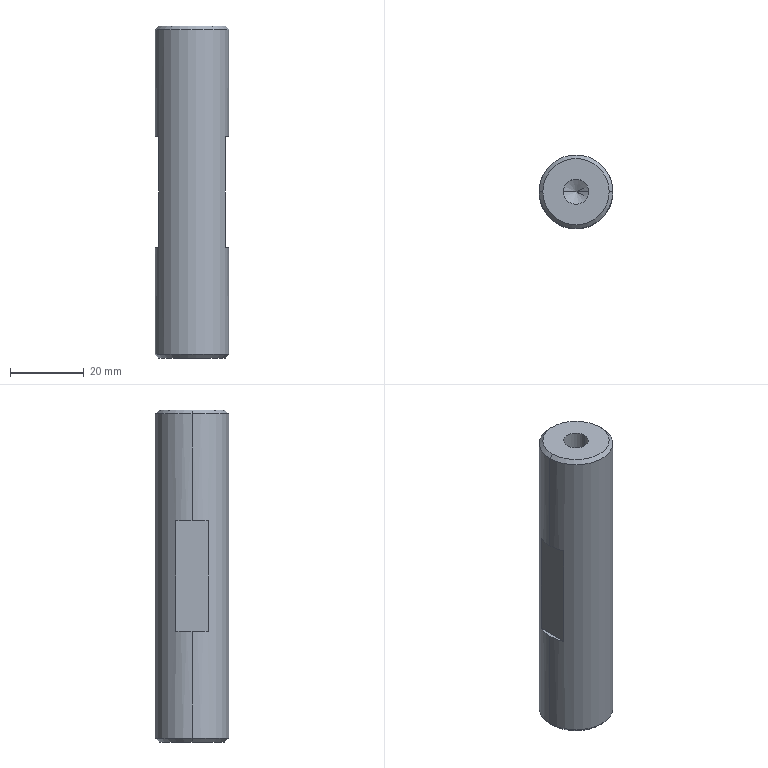Part | STEP file | 08-07 limit post | 1 solid | 22 faces | box 20 x 20 x 90 mm | volume 26377 mm3 | cone 8 | plane 8 | cylinder 6 | commonest cylinder face diameters 6.8 x4 20 x2
STEP:
#1=CARTESIAN_POINT('',(3.4,0.,19.75));
#2=VERTEX_POINT('',#1);
#3=CARTESIAN_POINT('',(-3.4,0.,19.75));
#4=VERTEX_POINT('',#3);
#5=CARTESIAN_POINT('',(0.,0.,19.75));
#6=DIRECTION('',(0.,0.,-1.));
#7=DIRECTION('',(-1.,0.,0.));
#8=AXIS2_PLACEMENT_3D('',#5,#6,#7);
#9=CIRCLE('',#8,3.4);
#10=EDGE_CURVE('',#2,#4,#9,.T.);
#11=ORIENTED_EDGE('',*,*,#10,.F.);
#12=CARTESIAN_POINT('',(3.4,0.,0.));
#13=VERTEX_POINT('',#12);
#14=CARTESIAN_POINT('',(3.4,0.,0.));
#15=DIRECTION('',(0.,0.,-1.));
#16=VECTOR('',#15,1000.);
#17=LINE('',#14,#16);
#18=EDGE_CURVE('',#2,#13,#17,.T.);
#19=ORIENTED_EDGE('',*,*,#18,.T.);
#20=CARTESIAN_POINT('',(-3.4,0.,0.));
#21=VERTEX_POINT('',#20);
#22=CARTESIAN_POINT('',(0.,0.,0.));
#23=DIRECTION('',(0.,0.,-1.));
#24=DIRECTION('',(-1.,0.,0.));
#25=AXIS2_PLACEMENT_3D('',#22,#23,#24);
#26=CIRCLE('',#25,3.4);
#27=EDGE_CURVE('',#13,#21,#26,.T.);
#28=ORIENTED_EDGE('',*,*,#27,.T.);
#29=CARTESIAN_POINT('',(-3.4,0.,0.));
#30=DIRECTION('',(0.,0.,-1.));
#31=VECTOR('',#30,1000.);
#32=LINE('',#29,#31);
#33=EDGE_CURVE('',#4,#21,#32,.T.);
#34=ORIENTED_EDGE('',*,*,#33,.F.);
#35=EDGE_LOOP('',(#11,#19,#28,#34));
#36=FACE_OUTER_BOUND('',#35,.T.);
#37=CARTESIAN_POINT('',(0.,0.,0.));
#38=DIRECTION('',(0.,0.,-1.));
#39=DIRECTION('',(-1.,0.,0.));
#40=AXIS2_PLACEMENT_3D('',#37,#38,#39);
#41=CYLINDRICAL_SURFACE('',#40,3.4);
#42=ADVANCED_FACE('',(#36),#41,.F.);
#43=CARTESIAN_POINT('',(0.,0.,21.793));
#44=VERTEX_POINT('',#43);
#45=CARTESIAN_POINT('',(-3.4,0.,19.75));
#46=DIRECTION('',(-0.8572,0.,-0.515));
#47=VECTOR('',#46,1000.);
#48=LINE('',#45,#47);
#49=EDGE_CURVE('',#44,#4,#48,.T.);
#50=ORIENTED_EDGE('',*,*,#49,.F.);
#51=CARTESIAN_POINT('',(3.4,0.,19.75));
#52=DIRECTION('',(0.8572,0.,-0.515));
#53=VECTOR('',#52,1000.);
#54=LINE('',#51,#53);
#55=EDGE_CURVE('',#44,#2,#54,.T.);
#56=ORIENTED_EDGE('',*,*,#55,.T.);
#57=ORIENTED_EDGE('',*,*,#10,.T.);
#58=EDGE_LOOP('',(#50,#56,#57));
#59=FACE_OUTER_BOUND('',#58,.T.);
#60=CARTESIAN_POINT('',(0.,0.,19.75));
#61=DIRECTION('',(0.,0.,-1.));
#62=DIRECTION('',(-1.,0.,0.));
#63=AXIS2_PLACEMENT_3D('',#60,#61,#62);
#64=CONICAL_SURFACE('',#63,3.4,1.03);
#65=ADVANCED_FACE('',(#59),#64,.F.);
#66=CARTESIAN_POINT('',(-3.4,0.,70.25));
#67=VERTEX_POINT('',#66);
#68=CARTESIAN_POINT('',(3.4,0.,70.25));
#69=VERTEX_POINT('',#68);
#70=CARTESIAN_POINT('',(0.,0.,70.25));
#71=DIRECTION('',(0.,0.,1.));
#72=DIRECTION('',(1.,0.,0.));
#73=AXIS2_PLACEMENT_3D('',#70,#71,#72);
#74=CIRCLE('',#73,3.4);
#75=EDGE_CURVE('',#67,#69,#74,.T.);
#76=ORIENTED_EDGE('',*,*,#75,.F.);
#77=CARTESIAN_POINT('',(-3.4,0.,90.));
#78=VERTEX_POINT('',#77);
#79=CARTESIAN_POINT('',(-3.4,0.,90.));
#80=DIRECTION('',(0.,0.,1.));
#81=VECTOR('',#80,1000.);
#82=LINE('',#79,#81);
#83=EDGE_CURVE('',#67,#78,#82,.T.);
#84=ORIENTED_EDGE('',*,*,#83,.T.);
#85=CARTESIAN_POINT('',(3.4,0.,90.));
#86=VERTEX_POINT('',#85);
#87=CARTESIAN_POINT('',(0.,0.,90.));
#88=DIRECTION('',(0.,0.,1.));
#89=DIRECTION('',(1.,0.,0.));
#90=AXIS2_PLACEMENT_3D('',#87,#88,#89);
#91=CIRCLE('',#90,3.4);
#92=EDGE_CURVE('',#78,#86,#91,.T.);
#93=ORIENTED_EDGE('',*,*,#92,.T.);
#94=CARTESIAN_POINT('',(3.4,0.,90.));
#95=DIRECTION('',(0.,0.,1.));
#96=VECTOR('',#95,1000.);
#97=LINE('',#94,#96);
#98=EDGE_CURVE('',#69,#86,#97,.T.);
#99=ORIENTED_EDGE('',*,*,#98,.F.);
#100=EDGE_LOOP('',(#76,#84,#93,#99));
#101=FACE_OUTER_BOUND('',#100,.T.);
#102=CARTESIAN_POINT('',(0.,0.,90.));
#103=DIRECTION('',(0.,0.,1.));
#104=DIRECTION('',(1.,0.,0.));
#105=AXIS2_PLACEMENT_3D('',#102,#103,#104);
#106=CYLINDRICAL_SURFACE('',#105,3.4);
#107=ADVANCED_FACE('',(#101),#106,.F.);
#108=CARTESIAN_POINT('',(0.,0.,68.207));
#109=VERTEX_POINT('',#108);
#110=CARTESIAN_POINT('',(3.4,0.,70.25));
#111=DIRECTION('',(0.8572,0.,0.515));
#112=VECTOR('',#111,1000.);
#113=LINE('',#110,#112);
#114=EDGE_CURVE('',#109,#69,#113,.T.);
#115=ORIENTED_EDGE('',*,*,#114,.F.);
#116=CARTESIAN_POINT('',(-3.4,0.,70.25));
#117=DIRECTION('',(-0.8572,0.,0.515));
#118=VECTOR('',#117,1000.);
#119=LINE('',#116,#118);
#120=EDGE_CURVE('',#109,#67,#119,.T.);
#121=ORIENTED_EDGE('',*,*,#120,.T.);
#122=ORIENTED_EDGE('',*,*,#75,.T.);
#123=EDGE_LOOP('',(#115,#121,#122));
#124=FACE_OUTER_BOUND('',#123,.T.);
#125=CARTESIAN_POINT('',(0.,0.,70.25));
#126=DIRECTION('',(0.,0.,1.));
#127=DIRECTION('',(1.,0.,0.));
#128=AXIS2_PLACEMENT_3D('',#125,#126,#127);
#129=CONICAL_SURFACE('',#128,3.4,1.03);
#130=ADVANCED_FACE('',(#124),#129,.F.);
#131=CARTESIAN_POINT('',(9.,0.,90.));
#132=VERTEX_POINT('',#131);
#133=CARTESIAN_POINT('',(-9.,0.,90.));
#134=VERTEX_POINT('',#133);
#135=CARTESIAN_POINT('',(0.,0.,90.));
#136=DIRECTION('',(0.,0.,1.));
#137=DIRECTION('',(1.,0.,0.));
#138=AXIS2_PLACEMENT_3D('',#135,#136,#137);
#139=CIRCLE('',#138,9.);
#140=EDGE_CURVE('',#132,#134,#139,.T.);
#141=ORIENTED_EDGE('',*,*,#140,.F.);
#142=CARTESIAN_POINT('',(10.,0.,89.));
#143=VERTEX_POINT('',#142);
#144=CARTESIAN_POINT('',(9.,0.,90.));
#145=DIRECTION('',(0.7071,0.,-0.7071));
#146=VECTOR('',#145,1000.);
#147=LINE('',#144,#146);
#148=EDGE_CURVE('',#132,#143,#147,.T.);
#149=ORIENTED_EDGE('',*,*,#148,.T.);
#150=CARTESIAN_POINT('',(-10.,0.,89.));
#151=VERTEX_POINT('',#150);
#152=CARTESIAN_POINT('',(0.,0.,89.));
#153=DIRECTION('',(0.,0.,-1.));
#154=DIRECTION('',(1.,0.,0.));
#155=AXIS2_PLACEMENT_3D('',#152,#153,#154);
#156=CIRCLE('',#155,10.);
#157=EDGE_CURVE('',#151,#143,#156,.T.);
#158=ORIENTED_EDGE('',*,*,#157,.F.);
#159=CARTESIAN_POINT('',(-9.,0.,90.));
#160=DIRECTION('',(-0.7071,0.,-0.7071));
#161=VECTOR('',#160,1000.);
#162=LINE('',#159,#161);
#163=EDGE_CURVE('',#134,#151,#162,.T.);
#164=ORIENTED_EDGE('',*,*,#163,.F.);
#165=EDGE_LOOP('',(#141,#149,#158,#164));
#166=FACE_OUTER_BOUND('',#165,.T.);
#167=CARTESIAN_POINT('',(0.,0.,90.));
#168=DIRECTION('',(0.,0.,-1.));
#169=DIRECTION('',(-1.,0.,0.));
#170=AXIS2_PLACEMENT_3D('',#167,#168,#169);
#171=CONICAL_SURFACE('',#170,9.,0.7854);
#172=ADVANCED_FACE('',(#166),#171,.T.);
#173=CARTESIAN_POINT('',(-9.,0.,0.));
#174=VERTEX_POINT('',#173);
#175=CARTESIAN_POINT('',(9.,0.,0.));
#176=VERTEX_POINT('',#175);
#177=CARTESIAN_POINT('',(0.,0.,0.));
#178=DIRECTION('',(0.,0.,-1.));
#179=DIRECTION('',(1.,0.,0.));
#180=AXIS2_PLACEMENT_3D('',#177,#178,#179);
#181=CIRCLE('',#180,9.);
#182=EDGE_CURVE('',#174,#176,#181,.T.);
#183=ORIENTED_EDGE('',*,*,#182,.F.);
#184=CARTESIAN_POINT('',(-10.,0.,1.));
#185=VERTEX_POINT('',#184);
#186=CARTESIAN_POINT('',(-10.,0.,1.));
#187=DIRECTION('',(-0.7071,0.,0.7071));
#188=VECTOR('',#187,1000.);
#189=LINE('',#186,#188);
#190=EDGE_CURVE('',#174,#185,#189,.T.);
#191=ORIENTED_EDGE('',*,*,#190,.T.);
#192=CARTESIAN_POINT('',(10.,0.,1.));
#193=VERTEX_POINT('',#192);
#194=CARTESIAN_POINT('',(0.,0.,1.));
#195=DIRECTION('',(0.,0.,1.));
#196=DIRECTION('',(1.,0.,0.));
#197=AXIS2_PLACEMENT_3D('',#194,#195,#196);
#198=CIRCLE('',#197,10.);
#199=EDGE_CURVE('',#193,#185,#198,.T.);
#200=ORIENTED_EDGE('',*,*,#199,.F.);
#201=CARTESIAN_POINT('',(10.,0.,1.));
#202=DIRECTION('',(0.7071,0.,0.7071));
#203=VECTOR('',#202,1000.);
#204=LINE('',#201,#203);
#205=EDGE_CURVE('',#176,#193,#204,.T.);
#206=ORIENTED_EDGE('',*,*,#205,.F.);
#207=EDGE_LOOP('',(#183,#191,#200,#206));
#208=FACE_OUTER_BOUND('',#207,.T.);
#209=CARTESIAN_POINT('',(0.,0.,1.));
#210=DIRECTION('',(0.,0.,1.));
#211=DIRECTION('',(1.,0.,0.));
#212=AXIS2_PLACEMENT_3D('',#209,#210,#211);
#213=CONICAL_SURFACE('',#212,10.,0.7854);
#214=ADVANCED_FACE('',(#208),#213,.T.);
#215=ORIENTED_EDGE('',*,*,#157,.T.);
#216=CARTESIAN_POINT('',(10.,0.,60.));
#217=VERTEX_POINT('',#216);
#218=CARTESIAN_POINT('',(10.,0.,90.));
#219=DIRECTION('',(0.,0.,-1.));
#220=VECTOR('',#219,1000.);
#221=LINE('',#218,#220);
#222=EDGE_CURVE('',#143,#217,#221,.T.);
#223=ORIENTED_EDGE('',*,*,#222,.T.);
#224=CARTESIAN_POINT('',(9.,4.359,60.));
#225=VERTEX_POINT('',#224);
#226=CARTESIAN_POINT('',(0.,0.,60.));
#227=DIRECTION('',(0.,0.,1.));
#228=DIRECTION('',(1.,0.,0.));
#229=AXIS2_PLACEMENT_3D('',#226,#227,#228);
#230=CIRCLE('',#229,10.);
#231=EDGE_CURVE('',#217,#225,#230,.T.);
#232=ORIENTED_EDGE('',*,*,#231,.T.);
#233=CARTESIAN_POINT('',(9.,4.359,30.));
#234=VERTEX_POINT('',#233);
#235=CARTESIAN_POINT('',(9.,4.359,90.));
#236=DIRECTION('',(0.,0.,-1.));
#237=VECTOR('',#236,1000.);
#238=LINE('',#235,#237);
#239=EDGE_CURVE('',#225,#234,#238,.T.);
#240=ORIENTED_EDGE('',*,*,#239,.T.);
#241=CARTESIAN_POINT('',(10.,0.,30.));
#242=VERTEX_POINT('',#241);
#243=CARTESIAN_POINT('',(0.,0.,30.));
#244=DIRECTION('',(0.,0.,-1.));
#245=DIRECTION('',(-1.,0.,0.));
#246=AXIS2_PLACEMENT_3D('',#243,#244,#245);
#247=CIRCLE('',#246,10.);
#248=EDGE_CURVE('',#234,#242,#247,.T.);
#249=ORIENTED_EDGE('',*,*,#248,.T.);
#250=CARTESIAN_POINT('',(10.,0.,90.));
#251=DIRECTION('',(0.,0.,-1.));
#252=VECTOR('',#251,1000.);
#253=LINE('',#250,#252);
#254=EDGE_CURVE('',#242,#193,#253,.T.);
#255=ORIENTED_EDGE('',*,*,#254,.T.);
#256=ORIENTED_EDGE('',*,*,#199,.T.);
#257=CARTESIAN_POINT('',(-10.,0.,30.));
#258=VERTEX_POINT('',#257);
#259=CARTESIAN_POINT('',(-10.,0.,90.));
#260=DIRECTION('',(0.,0.,-1.));
#261=VECTOR('',#260,1000.);
#262=LINE('',#259,#261);
#263=EDGE_CURVE('',#258,#185,#262,.T.);
#264=ORIENTED_EDGE('',*,*,#263,.F.);
#265=CARTESIAN_POINT('',(-9.,4.359,30.));
#266=VERTEX_POINT('',#265);
#267=CARTESIAN_POINT('',(0.,0.,30.));
#268=DIRECTION('',(0.,0.,-1.));
#269=DIRECTION('',(-1.,0.,0.));
#270=AXIS2_PLACEMENT_3D('',#267,#268,#269);
#271=CIRCLE('',#270,10.);
#272=EDGE_CURVE('',#258,#266,#271,.T.);
#273=ORIENTED_EDGE('',*,*,#272,.T.);
#274=CARTESIAN_POINT('',(-9.,4.359,60.));
#275=VERTEX_POINT('',#274);
#276=CARTESIAN_POINT('',(-9.,4.359,90.));
#277=DIRECTION('',(0.,0.,1.));
#278=VECTOR('',#277,1000.);
#279=LINE('',#276,#278);
#280=EDGE_CURVE('',#266,#275,#279,.T.);
#281=ORIENTED_EDGE('',*,*,#280,.T.);
#282=CARTESIAN_POINT('',(-10.,0.,60.));
#283=VERTEX_POINT('',#282);
#284=CARTESIAN_POINT('',(0.,0.,60.));
#285=DIRECTION('',(0.,0.,1.));
#286=DIRECTION('',(1.,0.,0.));
#287=AXIS2_PLACEMENT_3D('',#284,#285,#286);
#288=CIRCLE('',#287,10.);
#289=EDGE_CURVE('',#275,#283,#288,.T.);
#290=ORIENTED_EDGE('',*,*,#289,.T.);
#291=CARTESIAN_POINT('',(-10.,0.,90.));
#292=DIRECTION('',(0.,0.,-1.));
#293=VECTOR('',#292,1000.);
#294=LINE('',#291,#293);
#295=EDGE_CURVE('',#151,#283,#294,.T.);
#296=ORIENTED_EDGE('',*,*,#295,.F.);
#297=EDGE_LOOP('',(#215,#223,#232,#240,#249,#255,#256,#264,#273,#281,#290,#296));
#298=FACE_OUTER_BOUND('',#297,.T.);
#299=CARTESIAN_POINT('',(0.,0.,90.));
#300=DIRECTION('',(0.,0.,-1.));
#301=DIRECTION('',(-1.,0.,0.));
#302=AXIS2_PLACEMENT_3D('',#299,#300,#301);
#303=CYLINDRICAL_SURFACE('',#302,10.);
#304=ADVANCED_FACE('',(#298),#303,.T.);
#305=ORIENTED_EDGE('',*,*,#222,.F.);
#306=CARTESIAN_POINT('',(0.,0.,89.));
#307=DIRECTION('',(0.,0.,-1.));
#308=DIRECTION('',(1.,0.,0.));
#309=AXIS2_PLACEMENT_3D('',#306,#307,#308);
#310=CIRCLE('',#309,10.);
#311=EDGE_CURVE('',#143,#151,#310,.T.);
#312=ORIENTED_EDGE('',*,*,#311,.T.);
#313=ORIENTED_EDGE('',*,*,#295,.T.);
#314=CARTESIAN_POINT('',(-9.,-4.359,60.));
#315=VERTEX_POINT('',#314);
#316=CARTESIAN_POINT('',(0.,0.,60.));
#317=DIRECTION('',(0.,0.,1.));
#318=DIRECTION('',(1.,0.,0.));
#319=AXIS2_PLACEMENT_3D('',#316,#317,#318);
#320=CIRCLE('',#319,10.);
#321=EDGE_CURVE('',#283,#315,#320,.T.);
#322=ORIENTED_EDGE('',*,*,#321,.T.);
#323=CARTESIAN_POINT('',(-9.,-4.359,30.));
#324=VERTEX_POINT('',#323);
#325=CARTESIAN_POINT('',(-9.,-4.359,90.));
#326=DIRECTION('',(0.,0.,-1.));
#327=VECTOR('',#326,1000.);
#328=LINE('',#325,#327);
#329=EDGE_CURVE('',#315,#324,#328,.T.);
#330=ORIENTED_EDGE('',*,*,#329,.T.);
#331=CARTESIAN_POINT('',(0.,0.,30.));
#332=DIRECTION('',(0.,0.,-1.));
#333=DIRECTION('',(-1.,0.,0.));
#334=AXIS2_PLACEMENT_3D('',#331,#332,#333);
#335=CIRCLE('',#334,10.);
#336=EDGE_CURVE('',#324,#258,#335,.T.);
#337=ORIENTED_EDGE('',*,*,#336,.T.);
#338=ORIENTED_EDGE('',*,*,#263,.T.);
#339=CARTESIAN_POINT('',(0.,0.,1.));
#340=DIRECTION('',(0.,0.,1.));
#341=DIRECTION('',(1.,0.,0.));
#342=AXIS2_PLACEMENT_3D('',#339,#340,#341);
#343=CIRCLE('',#342,10.);
#344=EDGE_CURVE('',#185,#193,#343,.T.);
#345=ORIENTED_EDGE('',*,*,#344,.T.);
#346=ORIENTED_EDGE('',*,*,#254,.F.);
#347=CARTESIAN_POINT('',(9.,-4.359,30.));
#348=VERTEX_POINT('',#347);
#349=CARTESIAN_POINT('',(0.,0.,30.));
#350=DIRECTION('',(0.,0.,-1.));
#351=DIRECTION('',(-1.,0.,0.));
#352=AXIS2_PLACEMENT_3D('',#349,#350,#351);
#353=CIRCLE('',#352,10.);
#354=EDGE_CURVE('',#242,#348,#353,.T.);
#355=ORIENTED_EDGE('',*,*,#354,.T.);
#356=CARTESIAN_POINT('',(9.,-4.359,60.));
#357=VERTEX_POINT('',#356);
#358=CARTESIAN_POINT('',(9.,-4.359,90.));
#359=DIRECTION('',(0.,0.,1.));
#360=VECTOR('',#359,1000.);
#361=LINE('',#358,#360);
#362=EDGE_CURVE('',#348,#357,#361,.T.);
#363=ORIENTED_EDGE('',*,*,#362,.T.);
#364=CARTESIAN_POINT('',(0.,0.,60.));
#365=DIRECTION('',(0.,0.,1.));
#366=DIRECTION('',(1.,0.,0.));
#367=AXIS2_PLACEMENT_3D('',#364,#365,#366);
#368=CIRCLE('',#367,10.);
#369=EDGE_CURVE('',#357,#217,#368,.T.);
#370=ORIENTED_EDGE('',*,*,#369,.T.);
#371=EDGE_LOOP('',(#305,#312,#313,#322,#330,#337,#338,#345,#346,#355,#363,#370));
#372=FACE_OUTER_BOUND('',#371,.T.);
#373=CARTESIAN_POINT('',(0.,0.,90.));
#374=DIRECTION('',(0.,0.,-1.));
#375=DIRECTION('',(-1.,0.,0.));
#376=AXIS2_PLACEMENT_3D('',#373,#374,#375);
#377=CYLINDRICAL_SURFACE('',#376,10.);
#378=ADVANCED_FACE('',(#372),#377,.T.);
#379=CARTESIAN_POINT('',(0.,0.,90.));
#380=DIRECTION('',(0.,0.,1.));
#381=DIRECTION('',(1.,0.,0.));
#382=AXIS2_PLACEMENT_3D('',#379,#380,#381);
#383=CIRCLE('',#382,3.4);
#384=EDGE_CURVE('',#86,#78,#383,.T.);
#385=ORIENTED_EDGE('',*,*,#384,.F.);
#386=ORIENTED_EDGE('',*,*,#92,.F.);
#387=EDGE_LOOP('',(#385,#386));
#388=FACE_BOUND('',#387,.T.);
#389=CARTESIAN_POINT('',(0.,0.,90.));
#390=DIRECTION('',(0.,0.,1.));
#391=DIRECTION('',(1.,0.,0.));
#392=AXIS2_PLACEMENT_3D('',#389,#390,#391);
#393=CIRCLE('',#392,9.);
#394=EDGE_CURVE('',#134,#132,#393,.T.);
#395=ORIENTED_EDGE('',*,*,#394,.T.);
#396=ORIENTED_EDGE('',*,*,#140,.T.);
#397=EDGE_LOOP('',(#395,#396));
#398=FACE_OUTER_BOUND('',#397,.T.);
#399=CARTESIAN_POINT('',(0.,0.,90.));
#400=DIRECTION('',(0.,0.,1.));
#401=DIRECTION('',(1.,0.,0.));
#402=AXIS2_PLACEMENT_3D('',#399,#400,#401);
#403=PLANE('',#402);
#404=ADVANCED_FACE('',(#388,#398),#403,.T.);
#405=CARTESIAN_POINT('',(0.,0.,0.));
#406=DIRECTION('',(0.,0.,-1.));
#407=DIRECTION('',(-1.,0.,0.));
#408=AXIS2_PLACEMENT_3D('',#405,#406,#407);
#409=CIRCLE('',#408,3.4);
#410=EDGE_CURVE('',#21,#13,#409,.T.);
#411=ORIENTED_EDGE('',*,*,#410,.F.);
#412=ORIENTED_EDGE('',*,*,#27,.F.);
#413=EDGE_LOOP('',(#411,#412));
#414=FACE_BOUND('',#413,.T.);
#415=CARTESIAN_POINT('',(0.,0.,0.));
#416=DIRECTION('',(0.,0.,-1.));
#417=DIRECTION('',(1.,0.,0.));
#418=AXIS2_PLACEMENT_3D('',#415,#416,#417);
#419=CIRCLE('',#418,9.);
#420=EDGE_CURVE('',#176,#174,#419,.T.);
#421=ORIENTED_EDGE('',*,*,#420,.T.);
#422=ORIENTED_EDGE('',*,*,#182,.T.);
#423=EDGE_LOOP('',(#421,#422));
#424=FACE_OUTER_BOUND('',#423,.T.);
#425=CARTESIAN_POINT('',(0.,0.,0.));
#426=DIRECTION('',(0.,0.,1.));
#427=DIRECTION('',(1.,0.,0.));
#428=AXIS2_PLACEMENT_3D('',#425,#426,#427);
#429=PLANE('',#428);
#430=ADVANCED_FACE('',(#414,#424),#429,.F.);
#431=ORIENTED_EDGE('',*,*,#190,.F.);
#432=ORIENTED_EDGE('',*,*,#420,.F.);
#433=ORIENTED_EDGE('',*,*,#205,.T.);
#434=ORIENTED_EDGE('',*,*,#344,.F.);
#435=EDGE_LOOP('',(#431,#432,#433,#434));
#436=FACE_OUTER_BOUND('',#435,.T.);
#437=CARTESIAN_POINT('',(0.,0.,1.));
#438=DIRECTION('',(0.,0.,1.));
#439=DIRECTION('',(1.,0.,0.));
#440=AXIS2_PLACEMENT_3D('',#437,#438,#439);
#441=CONICAL_SURFACE('',#440,10.,0.7854);
#442=ADVANCED_FACE('',(#436),#441,.T.);
#443=ORIENTED_EDGE('',*,*,#148,.F.);
#444=ORIENTED_EDGE('',*,*,#394,.F.);
#445=ORIENTED_EDGE('',*,*,#163,.T.);
#446=ORIENTED_EDGE('',*,*,#311,.F.);
#447=EDGE_LOOP('',(#443,#444,#445,#446));
#448=FACE_OUTER_BOUND('',#447,.T.);
#449=CARTESIAN_POINT('',(0.,0.,90.));
#450=DIRECTION('',(0.,0.,-1.));
#451=DIRECTION('',(-1.,0.,0.));
#452=AXIS2_PLACEMENT_3D('',#449,#450,#451);
#453=CONICAL_SURFACE('',#452,9.,0.7854);
#454=ADVANCED_FACE('',(#448),#453,.T.);
#455=ORIENTED_EDGE('',*,*,#120,.F.);
#456=ORIENTED_EDGE('',*,*,#114,.T.);
#457=CARTESIAN_POINT('',(0.,0.,70.25));
#458=DIRECTION('',(0.,0.,1.));
#459=DIRECTION('',(1.,0.,0.));
#460=AXIS2_PLACEMENT_3D('',#457,#458,#459);
#461=CIRCLE('',#460,3.4);
#462=EDGE_CURVE('',#69,#67,#461,.T.);
#463=ORIENTED_EDGE('',*,*,#462,.T.);
#464=EDGE_LOOP('',(#455,#456,#463));
#465=FACE_OUTER_BOUND('',#464,.T.);
#466=CARTESIAN_POINT('',(0.,0.,70.25));
#467=DIRECTION('',(0.,0.,1.));
#468=DIRECTION('',(1.,0.,0.));
#469=AXIS2_PLACEMENT_3D('',#466,#467,#468);
#470=CONICAL_SURFACE('',#469,3.4,1.03);
#471=ADVANCED_FACE('',(#465),#470,.F.);
#472=ORIENTED_EDGE('',*,*,#83,.F.);
#473=ORIENTED_EDGE('',*,*,#462,.F.);
#474=ORIENTED_EDGE('',*,*,#98,.T.);
#475=ORIENTED_EDGE('',*,*,#384,.T.);
#476=EDGE_LOOP('',(#472,#473,#474,#475));
#477=FACE_OUTER_BOUND('',#476,.T.);
#478=CARTESIAN_POINT('',(0.,0.,90.));
#479=DIRECTION('',(0.,0.,1.));
#480=DIRECTION('',(1.,0.,0.));
#481=AXIS2_PLACEMENT_3D('',#478,#479,#480);
#482=CYLINDRICAL_SURFACE('',#481,3.4);
#483=ADVANCED_FACE('',(#477),#482,.F.);
#484=ORIENTED_EDGE('',*,*,#55,.F.);
#485=ORIENTED_EDGE('',*,*,#49,.T.);
#486=CARTESIAN_POINT('',(0.,0.,19.75));
#487=DIRECTION('',(0.,0.,-1.));
#488=DIRECTION('',(-1.,0.,0.));
#489=AXIS2_PLACEMENT_3D('',#486,#487,#488);
#490=CIRCLE('',#489,3.4);
#491=EDGE_CURVE('',#4,#2,#490,.T.);
#492=ORIENTED_EDGE('',*,*,#491,.T.);
#493=EDGE_LOOP('',(#484,#485,#492));
#494=FACE_OUTER_BOUND('',#493,.T.);
#495=CARTESIAN_POINT('',(0.,0.,19.75));
#496=DIRECTION('',(0.,0.,-1.));
#497=DIRECTION('',(-1.,0.,0.));
#498=AXIS2_PLACEMENT_3D('',#495,#496,#497);
#499=CONICAL_SURFACE('',#498,3.4,1.03);
#500=ADVANCED_FACE('',(#494),#499,.F.);
#501=ORIENTED_EDGE('',*,*,#18,.F.);
#502=ORIENTED_EDGE('',*,*,#491,.F.);
#503=ORIENTED_EDGE('',*,*,#33,.T.);
#504=ORIENTED_EDGE('',*,*,#410,.T.);
#505=EDGE_LOOP('',(#501,#502,#503,#504));
#506=FACE_OUTER_BOUND('',#505,.T.);
#507=CARTESIAN_POINT('',(0.,0.,0.));
#508=DIRECTION('',(0.,0.,-1.));
#509=DIRECTION('',(-1.,0.,0.));
#510=AXIS2_PLACEMENT_3D('',#507,#508,#509);
#511=CYLINDRICAL_SURFACE('',#510,3.4);
#512=ADVANCED_FACE('',(#506),#511,.F.);
#513=CARTESIAN_POINT('',(9.,-5.,60.));
#514=DIRECTION('',(0.,1.,0.));
#515=VECTOR('',#514,1000.);
#516=LINE('',#513,#515);
#517=EDGE_CURVE('',#357,#225,#516,.T.);
#518=ORIENTED_EDGE('',*,*,#517,.F.);
#519=ORIENTED_EDGE('',*,*,#362,.F.);
#520=CARTESIAN_POINT('',(9.,-5.,30.));
#521=DIRECTION('',(0.,1.,0.));
#522=VECTOR('',#521,1000.);
#523=LINE('',#520,#522);
#524=EDGE_CURVE('',#348,#234,#523,.T.);
#525=ORIENTED_EDGE('',*,*,#524,.T.);
#526=ORIENTED_EDGE('',*,*,#239,.F.);
#527=EDGE_LOOP('',(#518,#519,#525,#526));
#528=FACE_OUTER_BOUND('',#527,.T.);
#529=CARTESIAN_POINT('',(9.,-5.,30.));
#530=DIRECTION('',(-1.,0.,0.));
#531=DIRECTION('',(0.,0.,1.));
#532=AXIS2_PLACEMENT_3D('',#529,#530,#531);
#533=PLANE('',#532);
#534=ADVANCED_FACE('',(#528),#533,.F.);
#535=ORIENTED_EDGE('',*,*,#524,.F.);
#536=ORIENTED_EDGE('',*,*,#354,.F.);
#537=ORIENTED_EDGE('',*,*,#248,.F.);
#538=EDGE_LOOP('',(#535,#536,#537));
#539=FACE_OUTER_BOUND('',#538,.T.);
#540=CARTESIAN_POINT('',(9.,-5.,30.));
#541=DIRECTION('',(0.,0.,-1.));
#542=DIRECTION('',(-1.,0.,0.));
#543=AXIS2_PLACEMENT_3D('',#540,#541,#542);
#544=PLANE('',#543);
#545=ADVANCED_FACE('',(#539),#544,.F.);
#546=ORIENTED_EDGE('',*,*,#517,.T.);
#547=ORIENTED_EDGE('',*,*,#231,.F.);
#548=ORIENTED_EDGE('',*,*,#369,.F.);
#549=EDGE_LOOP('',(#546,#547,#548));
#550=FACE_OUTER_BOUND('',#549,.T.);
#551=CARTESIAN_POINT('',(9.,-5.,60.));
#552=DIRECTION('',(0.,0.,1.));
#553=DIRECTION('',(1.,0.,0.));
#554=AXIS2_PLACEMENT_3D('',#551,#552,#553);
#555=PLANE('',#554);
#556=ADVANCED_FACE('',(#550),#555,.F.);
#557=CARTESIAN_POINT('',(-9.,-5.,30.));
#558=DIRECTION('',(0.,1.,0.));
#559=VECTOR('',#558,1000.);
#560=LINE('',#557,#559);
#561=EDGE_CURVE('',#324,#266,#560,.T.);
#562=ORIENTED_EDGE('',*,*,#561,.T.);
#563=ORIENTED_EDGE('',*,*,#272,.F.);
#564=ORIENTED_EDGE('',*,*,#336,.F.);
#565=EDGE_LOOP('',(#562,#563,#564));
#566=FACE_OUTER_BOUND('',#565,.T.);
#567=CARTESIAN_POINT('',(-9.,-5.,30.));
#568=DIRECTION('',(0.,0.,-1.));
#569=DIRECTION('',(-1.,0.,0.));
#570=AXIS2_PLACEMENT_3D('',#567,#568,#569);
#571=PLANE('',#570);
#572=ADVANCED_FACE('',(#566),#571,.F.);
#573=CARTESIAN_POINT('',(-9.,-5.,60.));
#574=DIRECTION('',(0.,1.,0.));
#575=VECTOR('',#574,1000.);
#576=LINE('',#573,#575);
#577=EDGE_CURVE('',#315,#275,#576,.T.);
#578=ORIENTED_EDGE('',*,*,#577,.T.);
#579=ORIENTED_EDGE('',*,*,#280,.F.);
#580=ORIENTED_EDGE('',*,*,#561,.F.);
#581=ORIENTED_EDGE('',*,*,#329,.F.);
#582=EDGE_LOOP('',(#578,#579,#580,#581));
#583=FACE_OUTER_BOUND('',#582,.T.);
#584=CARTESIAN_POINT('',(-9.,-5.,30.));
#585=DIRECTION('',(1.,0.,0.));
#586=DIRECTION('',(0.,0.,-1.));
#587=AXIS2_PLACEMENT_3D('',#584,#585,#586);
#588=PLANE('',#587);
#589=ADVANCED_FACE('',(#583),#588,.F.);
#590=ORIENTED_EDGE('',*,*,#577,.F.);
#591=ORIENTED_EDGE('',*,*,#321,.F.);
#592=ORIENTED_EDGE('',*,*,#289,.F.);
#593=EDGE_LOOP('',(#590,#591,#592));
#594=FACE_OUTER_BOUND('',#593,.T.);
#595=CARTESIAN_POINT('',(-9.,-5.,60.));
#596=DIRECTION('',(0.,0.,1.));
#597=DIRECTION('',(1.,0.,0.));
#598=AXIS2_PLACEMENT_3D('',#595,#596,#597);
#599=PLANE('',#598);
#600=ADVANCED_FACE('',(#594),#599,.F.);
#601=CLOSED_SHELL('',(#42,#65,#107,#130,#172,#214,#304,#378,#404,#430,#442,#454,#471,#483,#500,#512,#534,#545,#556,#572,#589,#600));
#602=MANIFOLD_SOLID_BREP('',#601);
#603=CARTESIAN_POINT('',(0.,0.,0.));
#604=DIRECTION('',(0.,0.,1.));
#605=DIRECTION('',(1.,0.,0.));
#606=AXIS2_PLACEMENT_3D('',#603,#604,#605);
#607=(LENGTH_UNIT()NAMED_UNIT(*)SI_UNIT(.MILLI.,.METRE.));
#608=UNCERTAINTY_MEASURE_WITH_UNIT(LENGTH_MEASURE(0.00001),#607,'','');
#609=(NAMED_UNIT(*)PLANE_ANGLE_UNIT()SI_UNIT($,.RADIAN.));
#610=(NAMED_UNIT(*)SI_UNIT($,.STERADIAN.)SOLID_ANGLE_UNIT());
#611=(GEOMETRIC_REPRESENTATION_CONTEXT(3)GLOBAL_UNCERTAINTY_ASSIGNED_CONTEXT((#608))GLOBAL_UNIT_ASSIGNED_CONTEXT((#607,#609,#610))REPRESENTATION_CONTEXT('',''));
#612=ADVANCED_BREP_SHAPE_REPRESENTATION('',(#602,#606),#611);